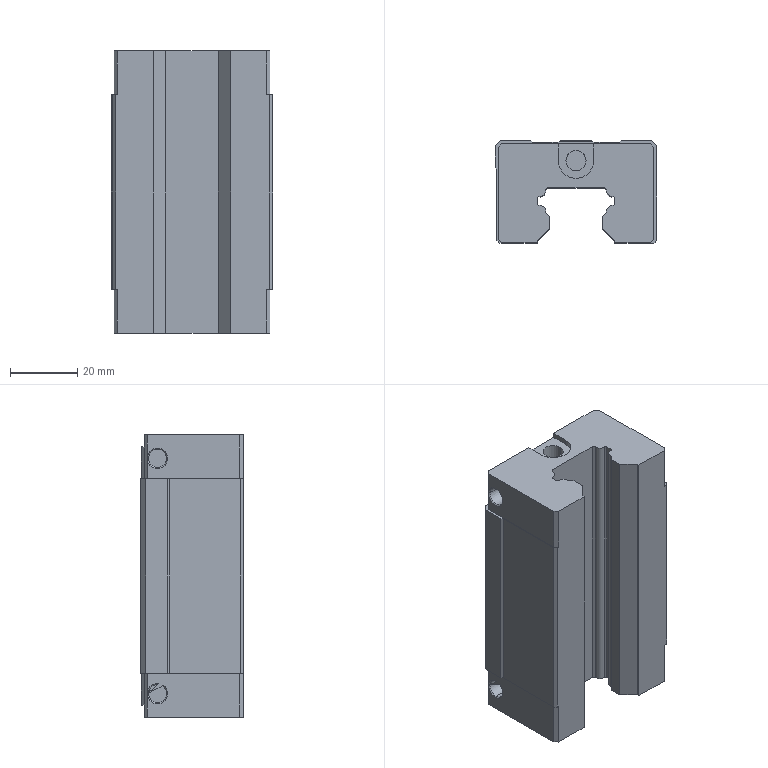Part | SolidWorks | features BaseBody 1 | 1 solid | 144 faces | box 48 x 30.5 x 84 mm | volume 91116 mm3 | plane 96 | cylinder 40 | cone 8 | commonest cylinder face diameters 6 x12 1 x8 5.4 x8 3.5 x6 7.3 x4 10.5 x2